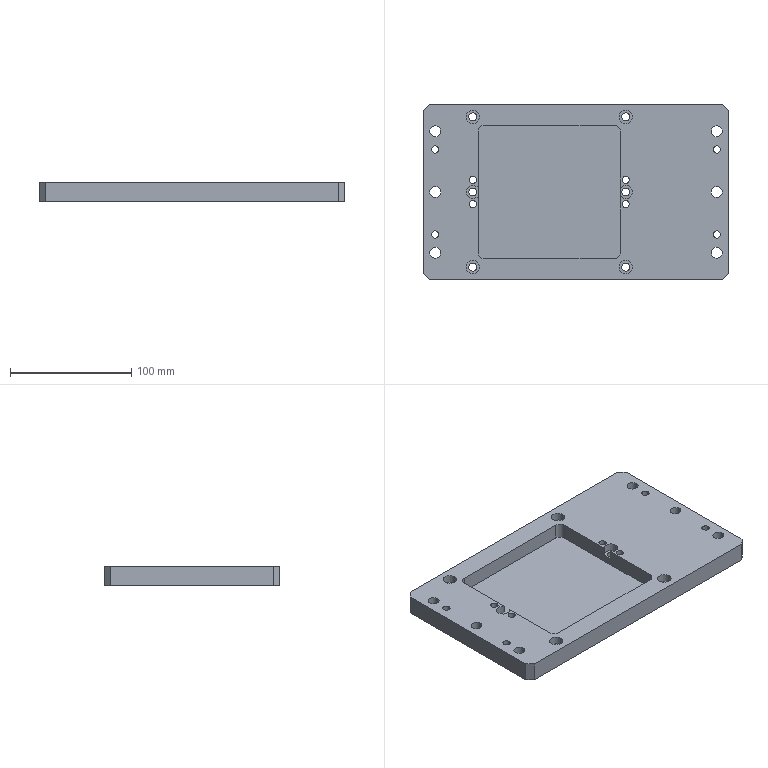Part | SolidWorks | features HoleWzd 5, Chamfer 1, Extrusion 1, ICE 1, MirrorPattern 1 | 1 solid | 102 faces | box 252 x 145 x 16 mm | volume 394345 mm3 | cylinder 71 | plane 27 | cone 4 | commonest cylinder face diameters 6 x16 6.6 x12 9 x12 15 x12 11 x11 5 x4